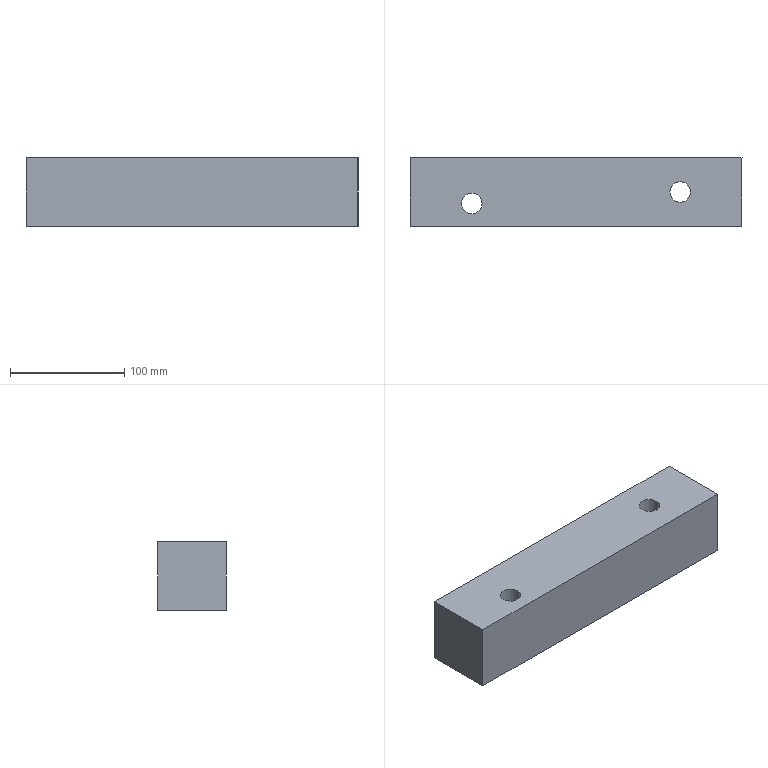Part | STEP file | lll_id542_x_t | 1 solid | 16 faces | box 290 x 60 x 60 mm | volume 989095 mm3 | plane 8 | cylinder 6 | cone 2 | commonest cylinder face diameters 14.506 x2 18.009 x2 26.007 x2
STEP:
#1=CARTESIAN_POINT('',(1960.182,640.,162.5));
#2=VERTEX_POINT('',#1);
#3=CARTESIAN_POINT('',(1967.435,640.,162.5));
#4=DIRECTION('',(0.,0.,1.));
#5=DIRECTION('',(-1.,0.,0.));
#6=AXIS2_PLACEMENT_3D('',#3,#4,#5);
#7=CIRCLE('',#6,7.253);
#8=EDGE_CURVE('',#2,#2,#7,.T.);
#9=ORIENTED_EDGE('',*,*,#8,.T.);
#10=EDGE_LOOP('',(#9));
#11=FACE_BOUND('',#10,.T.);
#12=CARTESIAN_POINT('',(2210.182,640.,162.5));
#13=VERTEX_POINT('',#12);
#14=CARTESIAN_POINT('',(2217.435,640.,162.5));
#15=DIRECTION('',(0.,0.,1.));
#16=DIRECTION('',(-1.,0.,0.));
#17=AXIS2_PLACEMENT_3D('',#14,#15,#16);
#18=CIRCLE('',#17,7.253);
#19=EDGE_CURVE('',#13,#13,#18,.T.);
#20=ORIENTED_EDGE('',*,*,#19,.T.);
#21=EDGE_LOOP('',(#20));
#22=FACE_BOUND('',#21,.T.);
#23=CARTESIAN_POINT('',(1947.435,600.,162.5));
#24=VERTEX_POINT('',#23);
#25=CARTESIAN_POINT('',(2237.435,600.,162.5));
#26=VERTEX_POINT('',#25);
#27=CARTESIAN_POINT('',(2052.435,600.,162.5));
#28=DIRECTION('',(1.,0.,0.));
#29=VECTOR('',#28,1.);
#30=LINE('',#27,#29);
#31=EDGE_CURVE('',#24,#26,#30,.T.);
#32=ORIENTED_EDGE('',*,*,#31,.F.);
#33=CARTESIAN_POINT('',(1947.435,660.,162.5));
#34=VERTEX_POINT('',#33);
#35=CARTESIAN_POINT('',(1947.435,631.,162.5));
#36=DIRECTION('',(0.,1.,0.));
#37=VECTOR('',#36,1.);
#38=LINE('',#35,#37);
#39=EDGE_CURVE('',#24,#34,#38,.T.);
#40=ORIENTED_EDGE('',*,*,#39,.T.);
#41=CARTESIAN_POINT('',(2237.435,660.,162.5));
#42=VERTEX_POINT('',#41);
#43=CARTESIAN_POINT('',(2211.935,660.,162.5));
#44=DIRECTION('',(1.,0.,0.));
#45=VECTOR('',#44,1.);
#46=LINE('',#43,#45);
#47=EDGE_CURVE('',#34,#42,#46,.T.);
#48=ORIENTED_EDGE('',*,*,#47,.T.);
#49=CARTESIAN_POINT('',(2237.435,582.5,162.5));
#50=DIRECTION('',(0.,1.,0.));
#51=VECTOR('',#50,1.);
#52=LINE('',#49,#51);
#53=EDGE_CURVE('',#26,#42,#52,.T.);
#54=ORIENTED_EDGE('',*,*,#53,.F.);
#55=EDGE_LOOP('',(#32,#40,#48,#54));
#56=FACE_BOUND('',#55,.T.);
#57=CARTESIAN_POINT('',(2014.439,620.,162.5));
#58=VERTEX_POINT('',#57);
#59=CARTESIAN_POINT('',(2001.435,620.,162.5));
#60=DIRECTION('',(0.,0.,1.));
#61=DIRECTION('',(1.,0.,0.));
#62=AXIS2_PLACEMENT_3D('',#59,#60,#61);
#63=CIRCLE('',#62,13.004);
#64=EDGE_CURVE('',#58,#58,#63,.T.);
#65=ORIENTED_EDGE('',*,*,#64,.T.);
#66=EDGE_LOOP('',(#65));
#67=FACE_BOUND('',#66,.T.);
#68=CARTESIAN_POINT('',(2170.432,630.,162.5));
#69=VERTEX_POINT('',#68);
#70=CARTESIAN_POINT('',(2183.435,630.,162.5));
#71=DIRECTION('',(0.,0.,-1.));
#72=DIRECTION('',(-1.,0.,0.));
#73=AXIS2_PLACEMENT_3D('',#70,#71,#72);
#74=CIRCLE('',#73,13.004);
#75=EDGE_CURVE('',#69,#69,#74,.T.);
#76=ORIENTED_EDGE('',*,*,#75,.F.);
#77=EDGE_LOOP('',(#76));
#78=FACE_BOUND('',#77,.T.);
#79=CARTESIAN_POINT('',(2092.435,582.5,162.5));
#80=DIRECTION('',(0.,0.,1.));
#81=DIRECTION('',(-1.,0.,0.));
#82=AXIS2_PLACEMENT_3D('',#79,#80,#81);
#83=PLANE('',#82);
#84=ADVANCED_FACE('',(#11,#22,#56,#67,#78),#83,.F.);
#85=CARTESIAN_POINT('',(2174.431,630.,222.5));
#86=VERTEX_POINT('',#85);
#87=CARTESIAN_POINT('',(2183.435,630.,222.5));
#88=DIRECTION('',(0.,0.,-1.));
#89=DIRECTION('',(-1.,0.,0.));
#90=AXIS2_PLACEMENT_3D('',#87,#88,#89);
#91=CIRCLE('',#90,9.005);
#92=EDGE_CURVE('',#86,#86,#91,.T.);
#93=ORIENTED_EDGE('',*,*,#92,.T.);
#94=EDGE_LOOP('',(#93));
#95=FACE_BOUND('',#94,.T.);
#96=CARTESIAN_POINT('',(1992.431,620.,222.5));
#97=VERTEX_POINT('',#96);
#98=CARTESIAN_POINT('',(2001.435,620.,222.5));
#99=DIRECTION('',(0.,0.,-1.));
#100=DIRECTION('',(-1.,0.,0.));
#101=AXIS2_PLACEMENT_3D('',#98,#99,#100);
#102=CIRCLE('',#101,9.005);
#103=EDGE_CURVE('',#97,#97,#102,.T.);
#104=ORIENTED_EDGE('',*,*,#103,.T.);
#105=EDGE_LOOP('',(#104));
#106=FACE_BOUND('',#105,.T.);
#107=CARTESIAN_POINT('',(2237.435,600.,222.5));
#108=VERTEX_POINT('',#107);
#109=CARTESIAN_POINT('',(2237.435,660.,222.5));
#110=VERTEX_POINT('',#109);
#111=CARTESIAN_POINT('',(2237.435,551.,222.5));
#112=DIRECTION('',(0.,1.,0.));
#113=VECTOR('',#112,1.);
#114=LINE('',#111,#113);
#115=EDGE_CURVE('',#108,#110,#114,.T.);
#116=ORIENTED_EDGE('',*,*,#115,.T.);
#117=CARTESIAN_POINT('',(1947.435,660.,222.5));
#118=VERTEX_POINT('',#117);
#119=CARTESIAN_POINT('',(2052.435,660.,222.5));
#120=DIRECTION('',(1.,0.,0.));
#121=VECTOR('',#120,1.);
#122=LINE('',#119,#121);
#123=EDGE_CURVE('',#118,#110,#122,.T.);
#124=ORIENTED_EDGE('',*,*,#123,.F.);
#125=CARTESIAN_POINT('',(1947.435,600.,222.5));
#126=VERTEX_POINT('',#125);
#127=CARTESIAN_POINT('',(1947.435,0.,222.5));
#128=DIRECTION('',(0.,1.,0.));
#129=VECTOR('',#128,1.);
#130=LINE('',#127,#129);
#131=EDGE_CURVE('',#126,#118,#130,.T.);
#132=ORIENTED_EDGE('',*,*,#131,.F.);
#133=CARTESIAN_POINT('',(2052.435,600.,222.5));
#134=DIRECTION('',(1.,0.,0.));
#135=VECTOR('',#134,1.);
#136=LINE('',#133,#135);
#137=EDGE_CURVE('',#126,#108,#136,.T.);
#138=ORIENTED_EDGE('',*,*,#137,.T.);
#139=EDGE_LOOP('',(#116,#124,#132,#138));
#140=FACE_BOUND('',#139,.T.);
#141=CARTESIAN_POINT('',(2052.435,0.,222.5));
#142=DIRECTION('',(0.,0.,1.));
#143=DIRECTION('',(-1.,0.,0.));
#144=AXIS2_PLACEMENT_3D('',#141,#142,#143);
#145=PLANE('',#144);
#146=ADVANCED_FACE('',(#95,#106,#140),#145,.T.);
#147=CARTESIAN_POINT('',(1947.435,660.,76.5));
#148=DIRECTION('',(0.,0.000000092,1.));
#149=VECTOR('',#148,1.);
#150=LINE('',#147,#149);
#151=EDGE_CURVE('',#34,#118,#150,.T.);
#152=ORIENTED_EDGE('',*,*,#151,.T.);
#153=ORIENTED_EDGE('',*,*,#123,.T.);
#154=CARTESIAN_POINT('',(2237.435,660.,76.5));
#155=DIRECTION('',(0.,0.000000092,1.));
#156=VECTOR('',#155,1.);
#157=LINE('',#154,#156);
#158=EDGE_CURVE('',#42,#110,#157,.T.);
#159=ORIENTED_EDGE('',*,*,#158,.F.);
#160=ORIENTED_EDGE('',*,*,#47,.F.);
#161=EDGE_LOOP('',(#152,#153,#159,#160));
#162=FACE_OUTER_BOUND('',#161,.T.);
#163=CARTESIAN_POINT('',(2211.935,660.,76.5));
#164=DIRECTION('',(0.,-1.,0.000000092));
#165=DIRECTION('',(1.,0.,0.));
#166=AXIS2_PLACEMENT_3D('',#163,#164,#165);
#167=PLANE('',#166);
#168=ADVANCED_FACE('',(#162),#167,.F.);
#169=ORIENTED_EDGE('',*,*,#53,.T.);
#170=ORIENTED_EDGE('',*,*,#158,.T.);
#171=ORIENTED_EDGE('',*,*,#115,.F.);
#172=CARTESIAN_POINT('',(2237.435,600.,142.5));
#173=DIRECTION('',(0.,0.,1.));
#174=VECTOR('',#173,1.);
#175=LINE('',#172,#174);
#176=EDGE_CURVE('',#26,#108,#175,.T.);
#177=ORIENTED_EDGE('',*,*,#176,.F.);
#178=EDGE_LOOP('',(#169,#170,#171,#177));
#179=FACE_OUTER_BOUND('',#178,.T.);
#180=CARTESIAN_POINT('',(2237.435,551.,76.5));
#181=DIRECTION('',(-1.,0.,0.));
#182=DIRECTION('',(0.,-0.000000092,-1.));
#183=AXIS2_PLACEMENT_3D('',#180,#181,#182);
#184=PLANE('',#183);
#185=ADVANCED_FACE('',(#179),#184,.F.);
#186=ORIENTED_EDGE('',*,*,#131,.T.);
#187=ORIENTED_EDGE('',*,*,#151,.F.);
#188=ORIENTED_EDGE('',*,*,#39,.F.);
#189=CARTESIAN_POINT('',(1947.435,600.,76.5));
#190=DIRECTION('',(0.,0.,1.));
#191=VECTOR('',#190,1.);
#192=LINE('',#189,#191);
#193=EDGE_CURVE('',#24,#126,#192,.T.);
#194=ORIENTED_EDGE('',*,*,#193,.T.);
#195=EDGE_LOOP('',(#186,#187,#188,#194));
#196=FACE_OUTER_BOUND('',#195,.T.);
#197=CARTESIAN_POINT('',(1947.435,631.,76.5));
#198=DIRECTION('',(1.,0.,0.));
#199=DIRECTION('',(0.,0.000000092,1.));
#200=AXIS2_PLACEMENT_3D('',#197,#198,#199);
#201=PLANE('',#200);
#202=ADVANCED_FACE('',(#196),#201,.F.);
#203=ORIENTED_EDGE('',*,*,#193,.F.);
#204=ORIENTED_EDGE('',*,*,#31,.T.);
#205=ORIENTED_EDGE('',*,*,#176,.T.);
#206=ORIENTED_EDGE('',*,*,#137,.F.);
#207=EDGE_LOOP('',(#203,#204,#205,#206));
#208=FACE_OUTER_BOUND('',#207,.T.);
#209=CARTESIAN_POINT('',(2052.435,600.,142.5));
#210=DIRECTION('',(0.,1.,0.));
#211=DIRECTION('',(0.,0.,-1.));
#212=AXIS2_PLACEMENT_3D('',#209,#210,#211);
#213=PLANE('',#212);
#214=ADVANCED_FACE('',(#208),#213,.F.);
#215=ORIENTED_EDGE('',*,*,#103,.F.);
#216=EDGE_LOOP('',(#215));
#217=FACE_BOUND('',#216,.T.);
#218=CARTESIAN_POINT('',(2010.44,620.,182.5));
#219=VERTEX_POINT('',#218);
#220=CARTESIAN_POINT('',(2001.435,620.,182.5));
#221=DIRECTION('',(0.,0.,1.));
#222=DIRECTION('',(1.,0.,0.));
#223=AXIS2_PLACEMENT_3D('',#220,#221,#222);
#224=CIRCLE('',#223,9.005);
#225=EDGE_CURVE('',#219,#219,#224,.T.);
#226=ORIENTED_EDGE('',*,*,#225,.F.);
#227=EDGE_LOOP('',(#226));
#228=FACE_BOUND('',#227,.T.);
#229=CARTESIAN_POINT('',(2001.435,620.,157.5));
#230=DIRECTION('',(0.,0.,1.));
#231=DIRECTION('',(1.,0.,0.));
#232=AXIS2_PLACEMENT_3D('',#229,#230,#231);
#233=CYLINDRICAL_SURFACE('',#232,9.005);
#234=ADVANCED_FACE('',(#217,#228),#233,.F.);
#235=ORIENTED_EDGE('',*,*,#225,.T.);
#236=EDGE_LOOP('',(#235));
#237=FACE_BOUND('',#236,.T.);
#238=CARTESIAN_POINT('',(2014.439,620.,182.5));
#239=VERTEX_POINT('',#238);
#240=CARTESIAN_POINT('',(2001.435,620.,182.5));
#241=DIRECTION('',(0.,0.,1.));
#242=DIRECTION('',(1.,0.,0.));
#243=AXIS2_PLACEMENT_3D('',#240,#241,#242);
#244=CIRCLE('',#243,13.004);
#245=EDGE_CURVE('',#239,#239,#244,.T.);
#246=ORIENTED_EDGE('',*,*,#245,.F.);
#247=EDGE_LOOP('',(#246));
#248=FACE_BOUND('',#247,.T.);
#249=CARTESIAN_POINT('',(2001.435,620.,182.5));
#250=DIRECTION('',(0.,0.,1.));
#251=DIRECTION('',(1.,0.,0.));
#252=AXIS2_PLACEMENT_3D('',#249,#250,#251);
#253=PLANE('',#252);
#254=ADVANCED_FACE('',(#237,#248),#253,.F.);
#255=ORIENTED_EDGE('',*,*,#245,.T.);
#256=EDGE_LOOP('',(#255));
#257=FACE_BOUND('',#256,.T.);
#258=ORIENTED_EDGE('',*,*,#64,.F.);
#259=EDGE_LOOP('',(#258));
#260=FACE_BOUND('',#259,.T.);
#261=CARTESIAN_POINT('',(2001.435,620.,162.5));
#262=DIRECTION('',(0.,0.,1.));
#263=DIRECTION('',(1.,0.,0.));
#264=AXIS2_PLACEMENT_3D('',#261,#262,#263);
#265=CYLINDRICAL_SURFACE('',#264,13.004);
#266=ADVANCED_FACE('',(#257,#260),#265,.F.);
#267=ORIENTED_EDGE('',*,*,#92,.F.);
#268=EDGE_LOOP('',(#267));
#269=FACE_BOUND('',#268,.T.);
#270=CARTESIAN_POINT('',(2174.431,630.,182.5));
#271=VERTEX_POINT('',#270);
#272=CARTESIAN_POINT('',(2183.435,630.,182.5));
#273=DIRECTION('',(0.,0.,-1.));
#274=DIRECTION('',(-1.,0.,0.));
#275=AXIS2_PLACEMENT_3D('',#272,#273,#274);
#276=CIRCLE('',#275,9.005);
#277=EDGE_CURVE('',#271,#271,#276,.T.);
#278=ORIENTED_EDGE('',*,*,#277,.T.);
#279=EDGE_LOOP('',(#278));
#280=FACE_BOUND('',#279,.T.);
#281=CARTESIAN_POINT('',(2183.435,630.,157.5));
#282=DIRECTION('',(0.,0.,1.));
#283=DIRECTION('',(-1.,0.,0.));
#284=AXIS2_PLACEMENT_3D('',#281,#282,#283);
#285=CYLINDRICAL_SURFACE('',#284,9.005);
#286=ADVANCED_FACE('',(#269,#280),#285,.F.);
#287=ORIENTED_EDGE('',*,*,#277,.F.);
#288=EDGE_LOOP('',(#287));
#289=FACE_BOUND('',#288,.T.);
#290=CARTESIAN_POINT('',(2170.432,630.,182.5));
#291=VERTEX_POINT('',#290);
#292=CARTESIAN_POINT('',(2183.435,630.,182.5));
#293=DIRECTION('',(0.,0.,-1.));
#294=DIRECTION('',(-1.,0.,0.));
#295=AXIS2_PLACEMENT_3D('',#292,#293,#294);
#296=CIRCLE('',#295,13.004);
#297=EDGE_CURVE('',#291,#291,#296,.T.);
#298=ORIENTED_EDGE('',*,*,#297,.T.);
#299=EDGE_LOOP('',(#298));
#300=FACE_BOUND('',#299,.T.);
#301=CARTESIAN_POINT('',(2183.435,630.,182.5));
#302=DIRECTION('',(0.,0.,1.));
#303=DIRECTION('',(-1.,0.,0.));
#304=AXIS2_PLACEMENT_3D('',#301,#302,#303);
#305=PLANE('',#304);
#306=ADVANCED_FACE('',(#289,#300),#305,.F.);
#307=ORIENTED_EDGE('',*,*,#297,.F.);
#308=EDGE_LOOP('',(#307));
#309=FACE_BOUND('',#308,.T.);
#310=ORIENTED_EDGE('',*,*,#75,.T.);
#311=EDGE_LOOP('',(#310));
#312=FACE_BOUND('',#311,.T.);
#313=CARTESIAN_POINT('',(2183.435,630.,162.5));
#314=DIRECTION('',(0.,0.,1.));
#315=DIRECTION('',(-1.,0.,0.));
#316=AXIS2_PLACEMENT_3D('',#313,#314,#315);
#317=CYLINDRICAL_SURFACE('',#316,13.004);
#318=ADVANCED_FACE('',(#309,#312),#317,.F.);
#319=CARTESIAN_POINT('',(2210.182,640.,200.253));
#320=VERTEX_POINT('',#319);
#321=CARTESIAN_POINT('',(2217.435,640.,200.253));
#322=DIRECTION('',(0.,0.,1.));
#323=DIRECTION('',(-1.,0.,0.));
#324=AXIS2_PLACEMENT_3D('',#321,#322,#323);
#325=CIRCLE('',#324,7.253);
#326=EDGE_CURVE('',#320,#320,#325,.T.);
#327=ORIENTED_EDGE('',*,*,#326,.T.);
#328=EDGE_LOOP('',(#327));
#329=FACE_BOUND('',#328,.T.);
#330=ORIENTED_EDGE('',*,*,#19,.F.);
#331=EDGE_LOOP('',(#330));
#332=FACE_BOUND('',#331,.T.);
#333=CARTESIAN_POINT('',(2217.435,640.,162.5));
#334=DIRECTION('',(0.,0.,1.));
#335=DIRECTION('',(1.,0.,0.));
#336=AXIS2_PLACEMENT_3D('',#333,#334,#335);
#337=CYLINDRICAL_SURFACE('',#336,7.253);
#338=ADVANCED_FACE('',(#329,#332),#337,.F.);
#339=CARTESIAN_POINT('',(2217.435,640.,207.506));
#340=VERTEX_POINT('',#339);
#341=VERTEX_LOOP('',#340);
#342=FACE_BOUND('',#341,.T.);
#343=ORIENTED_EDGE('',*,*,#326,.F.);
#344=EDGE_LOOP('',(#343));
#345=FACE_BOUND('',#344,.T.);
#346=CARTESIAN_POINT('',(2217.435,640.,200.253));
#347=DIRECTION('',(0.,0.,-1.));
#348=DIRECTION('',(-1.,0.,0.));
#349=AXIS2_PLACEMENT_3D('',#346,#347,#348);
#350=CONICAL_SURFACE('',#349,7.253,45.);
#351=ADVANCED_FACE('',(#342,#345),#350,.F.);
#352=CARTESIAN_POINT('',(1960.182,640.,200.253));
#353=VERTEX_POINT('',#352);
#354=CARTESIAN_POINT('',(1967.435,640.,200.253));
#355=DIRECTION('',(0.,0.,1.));
#356=DIRECTION('',(-1.,0.,0.));
#357=AXIS2_PLACEMENT_3D('',#354,#355,#356);
#358=CIRCLE('',#357,7.253);
#359=EDGE_CURVE('',#353,#353,#358,.T.);
#360=ORIENTED_EDGE('',*,*,#359,.T.);
#361=EDGE_LOOP('',(#360));
#362=FACE_BOUND('',#361,.T.);
#363=ORIENTED_EDGE('',*,*,#8,.F.);
#364=EDGE_LOOP('',(#363));
#365=FACE_BOUND('',#364,.T.);
#366=CARTESIAN_POINT('',(1967.435,640.,162.5));
#367=DIRECTION('',(0.,0.,1.));
#368=DIRECTION('',(1.,0.,0.));
#369=AXIS2_PLACEMENT_3D('',#366,#367,#368);
#370=CYLINDRICAL_SURFACE('',#369,7.253);
#371=ADVANCED_FACE('',(#362,#365),#370,.F.);
#372=CARTESIAN_POINT('',(1967.435,640.,207.506));
#373=VERTEX_POINT('',#372);
#374=VERTEX_LOOP('',#373);
#375=FACE_BOUND('',#374,.T.);
#376=ORIENTED_EDGE('',*,*,#359,.F.);
#377=EDGE_LOOP('',(#376));
#378=FACE_BOUND('',#377,.T.);
#379=CARTESIAN_POINT('',(1967.435,640.,200.253));
#380=DIRECTION('',(0.,0.,-1.));
#381=DIRECTION('',(-1.,0.,0.));
#382=AXIS2_PLACEMENT_3D('',#379,#380,#381);
#383=CONICAL_SURFACE('',#382,7.253,45.);
#384=ADVANCED_FACE('',(#375,#378),#383,.F.);
#385=CLOSED_SHELL('',(#84,#146,#168,#185,#202,#214,#234,#254,#266,#286,#306,#318,#338,#351,#371,#384));
#386=MANIFOLD_SOLID_BREP('',#385);
#387=(LENGTH_UNIT()NAMED_UNIT(*)SI_UNIT(.MILLI.,.METRE.));
#388=UNCERTAINTY_MEASURE_WITH_UNIT(LENGTH_MEASURE(0.00002),#387,'','');
#389=(NAMED_UNIT(*)PLANE_ANGLE_UNIT()SI_UNIT($,.RADIAN.));
#390=PLANE_ANGLE_MEASURE_WITH_UNIT(PLANE_ANGLE_MEASURE(0.01745),#389);
#391=DIMENSIONAL_EXPONENTS(0.,0.,0.,0.,0.,0.,0.);
#392=(CONVERSION_BASED_UNIT('DEGREE',#390)NAMED_UNIT(#391)PLANE_ANGLE_UNIT());
#393=(NAMED_UNIT(*)SI_UNIT($,.STERADIAN.)SOLID_ANGLE_UNIT());
#394=(GEOMETRIC_REPRESENTATION_CONTEXT(3)GLOBAL_UNCERTAINTY_ASSIGNED_CONTEXT((#388))GLOBAL_UNIT_ASSIGNED_CONTEXT((#387,#392,#393))REPRESENTATION_CONTEXT('',''));
#395=ADVANCED_BREP_SHAPE_REPRESENTATION('',(#386),#394);